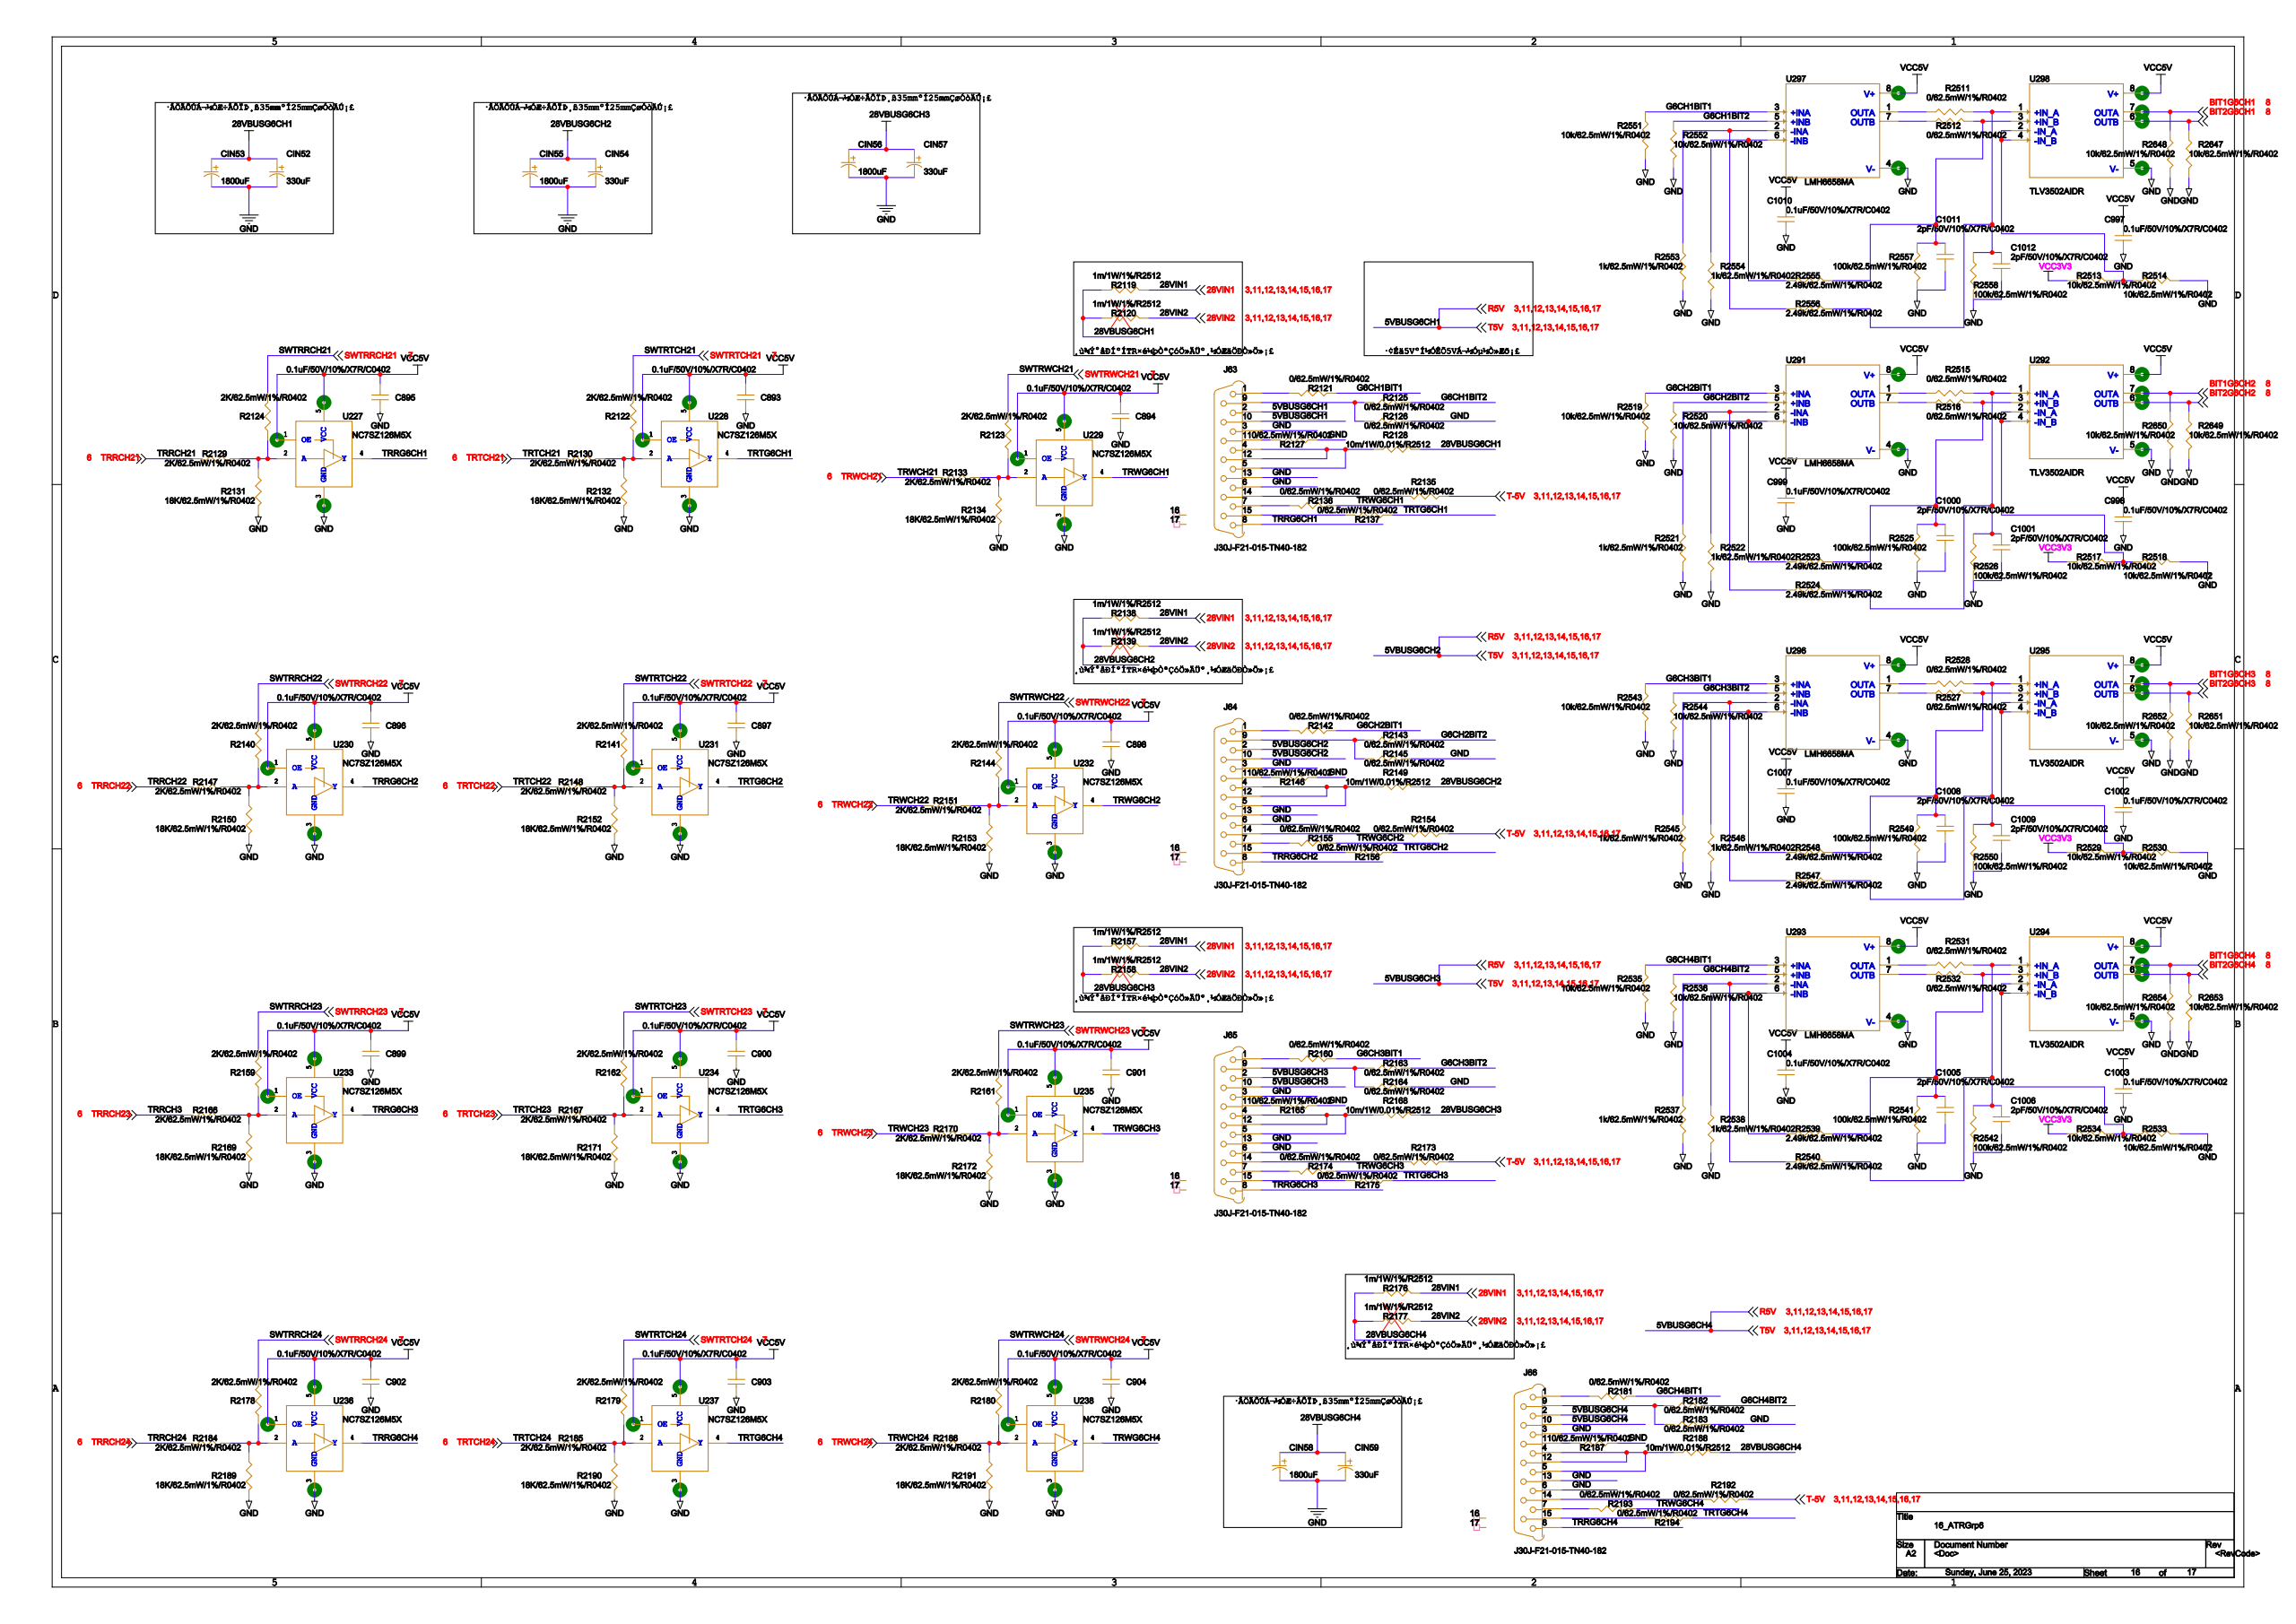Circuit board | Cadence Allegro | 1997 parts | 1536 nets | one sheet of the schematic
Parts on this sheet (reference | value | footprint):
C893 | 0.1uF/50V/10%/X7R/C0402 | 0402
C894 | 0.1uF/50V/10%/X7R/C0402 | 0402
C895 | 0.1uF/50V/10%/X7R/C0402 | 0402
C896 | 0.1uF/50V/10%/X7R/C0402 | 0402
C897 | 0.1uF/50V/10%/X7R/C0402 | 0402
C898 | 0.1uF/50V/10%/X7R/C0402 | 0402
C899 | 0.1uF/50V/10%/X7R/C0402 | 0402
C900 | 0.1uF/50V/10%/X7R/C0402 | 0402
C901 | 0.1uF/50V/10%/X7R/C0402 | 0402
C902 | 0.1uF/50V/10%/X7R/C0402 | 0402
C903 | 0.1uF/50V/10%/X7R/C0402 | 0402
C904 | 0.1uF/50V/10%/X7R/C0402 | 0402
C997 | 0.1uF/50V/10%/X7R/C0402 | 0402
C998 | 0.1uF/50V/10%/X7R/C0402 | 0402
C1000 | 2pF/50V/10%/X7R/C0402 | 0402
C1001 | 2pF/50V/10%/X7R/C0402 | 0402
C1002 | 0.1uF/50V/10%/X7R/C0402 | 0402
C1003 | 0.1uF/50V/10%/X7R/C0402 | 0402
C1005 | 2pF/50V/10%/X7R/C0402 | 0402
C1006 | 2pF/50V/10%/X7R/C0402 | 0402
C1008 | 2pF/50V/10%/X7R/C0402 | 0402
C1009 | 2pF/50V/10%/X7R/C0402 | 0402
C1011 | 2pF/50V/10%/X7R/C0402 | 0402
C1012 | 2pF/50V/10%/X7R/C0402 | 0402
CIN52 | ECF1JM331G20OTPO | AP-SMD_BD10-L20-W6_6-LS7_21
CIN53 | ECF1HM182M27OTPO | AP-SMD_BD18-L27-W6_6-LS7_21
CIN54 | ECF1JM331G20OTPO | AP-SMD_BD10-L20-W6_6-LS7_21
CIN55 | ECF1HM182M27OTPO | AP-SMD_BD18-L27-W6_6-LS7_21
CIN56 | ECF1HM182M27OTPO | AP-SMD_BD18-L27-W6_6-LS7_21
CIN57 | ECF1JM331G20OTPO | AP-SMD_BD10-L20-W6_6-LS7_21
CIN58 | ECF1HM182M27OTPO | AP-SMD_BD18-L27-W6_6-LS7_21
CIN59 | ECF1JM331G20OTPO | AP-SMD_BD10-L20-W6_6-LS7_21
J63 | J30J-F21-015-TN40-182 | J30J-F21-015-TN40-182
J64 | J30J-F21-015-TN40-182 | J30J-F21-015-TN40-182
J65 | J30J-F21-015-TN40-182 | J30J-F21-015-TN40-182
J66 | J30J-F21-015-TN40-182 | J30J-F21-015-TN40-182
R2119 | 1m/1W/1%/R2512 | 2512
R2120 | 1m/1W/1%/R2512 | 2512
R2121 | 0/62.5mW/1%/R0402 | 0402
R2122 | 2K/62.5mW/1%/R0402 | 0402
R2123 | 2K/62.5mW/1%/R0402 | 0402
R2124 | 2K/62.5mW/1%/R0402 | 0402
R2125 | 0/62.5mW/1%/R0402 | 0402
R2126 | 0/62.5mW/1%/R0402 | 0402
R2127 | 0/62.5mW/1%/R0402 | 0402
R2128 | 10m/1W/0.01%/R2512 | 2512
R2129 | 2K/62.5mW/1%/R0402 | 0402
R2130 | 2K/62.5mW/1%/R0402 | 0402
R2131 | 18K/62.5mW/1%/R0402 | 0402
R2132 | 18K/62.5mW/1%/R0402 | 0402
R2133 | 2K/62.5mW/1%/R0402 | 0402
R2134 | 18K/62.5mW/1%/R0402 | 0402
R2135 | 0/62.5mW/1%/R0402 | 0402
R2136 | 0/62.5mW/1%/R0402 | 0402
R2137 | 0/62.5mW/1%/R0402 | 0402
R2138 | 1m/1W/1%/R2512 | 2512
R2139 | 1m/1W/1%/R2512 | 2512
R2140 | 2K/62.5mW/1%/R0402 | 0402
R2141 | 2K/62.5mW/1%/R0402 | 0402
R2142 | 0/62.5mW/1%/R0402 | 0402
R2143 | 0/62.5mW/1%/R0402 | 0402
R2144 | 2K/62.5mW/1%/R0402 | 0402
R2145 | 0/62.5mW/1%/R0402 | 0402
R2146 | 0/62.5mW/1%/R0402 | 0402
R2147 | 2K/62.5mW/1%/R0402 | 0402
R2148 | 2K/62.5mW/1%/R0402 | 0402
R2149 | 10m/1W/0.01%/R2512 | 2512
R2150 | 18K/62.5mW/1%/R0402 | 0402
R2151 | 2K/62.5mW/1%/R0402 | 0402
R2152 | 18K/62.5mW/1%/R0402 | 0402
R2153 | 18K/62.5mW/1%/R0402 | 0402
R2154 | 0/62.5mW/1%/R0402 | 0402
R2155 | 0/62.5mW/1%/R0402 | 0402
R2156 | 0/62.5mW/1%/R0402 | 0402
R2157 | 1m/1W/1%/R2512 | 2512
R2158 | 1m/1W/1%/R2512 | 2512
R2159 | 2K/62.5mW/1%/R0402 | 0402
R2160 | 0/62.5mW/1%/R0402 | 0402
R2161 | 2K/62.5mW/1%/R0402 | 0402
R2162 | 2K/62.5mW/1%/R0402 | 0402
R2163 | 0/62.5mW/1%/R0402 | 0402
R2164 | 0/62.5mW/1%/R0402 | 0402
R2165 | 0/62.5mW/1%/R0402 | 0402
R2166 | 2K/62.5mW/1%/R0402 | 0402
R2167 | 2K/62.5mW/1%/R0402 | 0402
R2168 | 10m/1W/0.01%/R2512 | 2512
R2169 | 18K/62.5mW/1%/R0402 | 0402
R2170 | 2K/62.5mW/1%/R0402 | 0402
R2171 | 18K/62.5mW/1%/R0402 | 0402
R2172 | 18K/62.5mW/1%/R0402 | 0402
R2173 | 0/62.5mW/1%/R0402 | 0402
R2174 | 0/62.5mW/1%/R0402 | 0402
R2175 | 0/62.5mW/1%/R0402 | 0402
R2176 | 1m/1W/1%/R2512 | 2512
R2177 | 1m/1W/1%/R2512 | 2512
R2178 | 2K/62.5mW/1%/R0402 | 0402
R2179 | 2K/62.5mW/1%/R0402 | 0402
R2180 | 2K/62.5mW/1%/R0402 | 0402
R2181 | 0/62.5mW/1%/R0402 | 0402
R2182 | 0/62.5mW/1%/R0402 | 0402
R2183 | 0/62.5mW/1%/R0402 | 0402
R2184 | 2K/62.5mW/1%/R0402 | 0402
R2185 | 2K/62.5mW/1%/R0402 | 0402
R2186 | 2K/62.5mW/1%/R0402 | 0402
R2187 | 0/62.5mW/1%/R0402 | 0402
R2188 | 10m/1W/0.01%/R2512 | 2512
R2189 | 18K/62.5mW/1%/R0402 | 0402
R2190 | 18K/62.5mW/1%/R0402 | 0402
R2191 | 18K/62.5mW/1%/R0402 | 0402
R2192 | 0/62.5mW/1%/R0402 | 0402
R2193 | 0/62.5mW/1%/R0402 | 0402
R2194 | 0/62.5mW/1%/R0402 | 0402
R2511 | 0/62.5mW/1%/R0402 | 0402
R2512 | 0/62.5mW/1%/R0402 | 0402
R2513 | 10k/62.5mW/1%/R0402 | 0402
R2514 | 10k/62.5mW/1%/R0402 | 0402
R2515 | 0/62.5mW/1%/R0402 | 0402
R2516 | 0/62.5mW/1%/R0402 | 0402
R2517 | 10k/62.5mW/1%/R0402 | 0402
R2518 | 10k/62.5mW/1%/R0402 | 0402
R2519 | 10k/62.5mW/1%/R0402 | 0402
R2520 | 10k/62.5mW/1%/R0402 | 0402
R2521 | 1K/62.5mW/1%/R0402 | 0402
R2522 | 1K/62.5mW/1%/R0402 | 0402
R2524 | 2.49k/62.5mW/1%/R0402 | 0402
R2525 | 100k/62.5mW/1%/R0402 | 0402
R2526 | 100k/62.5mW/1%/R0402 | 0402
R2527 | 0/62.5mW/1%/R0402 | 0402
R2528 | 0/62.5mW/1%/R0402 | 0402
R2529 | 10k/62.5mW/1%/R0402 | 0402
R2530 | 10k/62.5mW/1%/R0402 | 0402
R2531 | 0/62.5mW/1%/R0402 | 0402
R2532 | 0/62.5mW/1%/R0402 | 0402
R2533 | 10k/62.5mW/1%/R0402 | 0402
R2534 | 10k/62.5mW/1%/R0402 | 0402
R2535 | 10k/62.5mW/1%/R0402 | 0402
R2536 | 10k/62.5mW/1%/R0402 | 0402
R2537 | 1K/62.5mW/1%/R0402 | 0402
R2538 | 1K/62.5mW/1%/R0402 | 0402
R2540 | 2.49k/62.5mW/1%/R0402 | 0402
R2541 | 100k/62.5mW/1%/R0402 | 0402
R2542 | 100k/62.5mW/1%/R0402 | 0402
R2543 | 10k/62.5mW/1%/R0402 | 0402
R2544 | 10k/62.5mW/1%/R0402 | 0402
R2545 | 1K/62.5mW/1%/R0402 | 0402
R2546 | 1K/62.5mW/1%/R0402 | 0402
R2547 | 2.49k/62.5mW/1%/R0402 | 0402
R2548 | 2.49k/62.5mW/1%/R0402 | 0402
R2549 | 100k/62.5mW/1%/R0402 | 0402
R2550 | 100k/62.5mW/1%/R0402 | 0402
R2551 | 10k/62.5mW/1%/R0402 | 0402
R2552 | 10k/62.5mW/1%/R0402 | 0402
R2553 | 1K/62.5mW/1%/R0402 | 0402
R2554 | 1K/62.5mW/1%/R0402 | 0402
R2556 | 2.49k/62.5mW/1%/R0402 | 0402
R2557 | 100k/62.5mW/1%/R0402 | 0402
R2558 | 100k/62.5mW/1%/R0402 | 0402
R2647 | 10k/62.5mW/1%/R0402 | 0402
R2648 | 10k/62.5mW/1%/R0402 | 0402
R2649 | 10k/62.5mW/1%/R0402 | 0402
R2650 | 10k/62.5mW/1%/R0402 | 0402
R2651 | 10k/62.5mW/1%/R0402 | 0402
R2652 | 10k/62.5mW/1%/R0402 | 0402
R2653 | 10k/62.5mW/1%/R0402 | 0402
R2654 | 10k/62.5mW/1%/R0402 | 0402
U227 | NC7SZ126M5X | SOT-23-5
U228 | NC7SZ126M5X | SOT-23-5
U229 | NC7SZ126M5X | SOT-23-5
U230 | NC7SZ126M5X | SOT-23-5
U231 | NC7SZ126M5X | SOT-23-5
U232 | NC7SZ126M5X | SOT-23-5
U233 | NC7SZ126M5X | SOT-23-5
U234 | NC7SZ126M5X | SOT-23-5
U235 | NC7SZ126M5X | SOT-23-5
U236 | NC7SZ126M5X | SOT-23-5
U237 | NC7SZ126M5X | SOT-23-5
U238 | NC7SZ126M5X | SOT-23-5
U291 | LMH6658MA | SOIC127P599X175-8N
U293 | LMH6658MA | SOIC127P599X175-8N
U295 | TLV3502AIDR | SOIC127P599X175-8N
U297 | LMH6658MA | SOIC127P599X175-8N
Nets of these parts (net: part-pin ...):
3.3V: R2513-1 R2517-1 R2529-1 R2534-1
AGND: C893-2 C894-2 C895-2 C896-2 C897-2 C898-2 C899-2 C900-2 C901-2 C902-2 C903-2 C904-2 C997-2 C998-2 C1000-2 C1001-2 C1002-2 C1003-2 C1005-2 C1006-2 C1008-2 C1009-2 C1011-2 C1012-2 CIN52-2 CIN53-2 CIN54-2 CIN55-2 CIN56-2 CIN57-2 CIN58-2 CIN59-2 J63-3 J63-6 J63-13 J64-3 J64-6 J64-13 J65-3 J65-6 J65-13 J66-3 J66-6 J66-13 R2126-1 R2127-1 R2131-1 R2132-1 R2134-1 R2145-1 R2146-1 R2150-1 R2152-1 R2153-1 R2164-1 R2165-1 R2169-1 R2171-1 R2172-1 R2183-1 R2187-1 R2189-1 R2190-1 R2191-1 R2514-2 R2518-2 R2519-2 R2520-2 R2521-2 R2522-2 R2525-2 R2526-2 R2530-2 R2533-2 R2535-2 R2536-2 R2537-2 R2538-2 R2541-2 R2542-2 R2543-2 R2544-2 R2545-2 R2546-2 R2549-2 R2550-2 R2551-2 R2552-2 R2553-2 R2554-2 R2557-2 R2558-2 R2647-2 R2648-2 R2649-2 R2650-2 R2651-2 R2652-2 R2653-2 R2654-2 U227-3 U228-3 U229-3 U230-3 U231-3 U232-3 U233-3 U234-3 U235-3 U236-3 U237-3 U238-3 U291-4 U293-4 U295-5 U297-4
VCC5V: C893-1 C894-1 C895-1 C896-1 C897-1 C898-1 C899-1 C900-1 C901-1 C902-1 C903-1 C904-1 C997-1 C998-1 C1002-1 C1003-1 U227-1 U227-5 U228-1 U228-5 U229-1 U229-5 U230-1 U230-5 U231-1 U231-5 U232-1 U232-5 U233-1 U233-5 U234-1 U234-5 U235-1 U235-5 U236-1 U236-5 U237-1 U237-5 U238-1 U238-5 U291-8 U293-8 U295-8 U297-8
N24409583: R2522-1 U291-6
N24409593: C1000-1 R2516-2 R2525-1
N24409571: R2521-1 R2524-1 U291-2
N24409591: C1001-1 R2515-2 R2524-2 R2526-1
N24410137: R2538-1 U293-6
N24410147: C1005-1 R2532-2 R2541-1
N24410125: R2537-1 R2540-1 U293-2
N24410145: C1006-1 R2531-2 R2540-2 R2542-1
N24409949: R2545-1 R2547-1
N24409965: C1009-1 R2528-2 R2547-2 R2550-1 U295-1
N24409953: R2546-1 R2548-1
N24409967: C1008-1 R2527-2 R2548-2 R2549-1 U295-3
N24409403: R2554-1 U297-6
N24409413: C1011-1 R2512-2 R2557-1
N24409399: R2553-1 R2556-1 U297-2
N24409411: C1012-1 R2511-2 R2556-2 R2558-1
G6CH2BIT1: R2142-1 R2519-1 U291-3
G6CH2BIT2: R2143-1 R2520-1 U291-5
N24409587: R2515-1 U291-1
N24409589: R2516-1 U291-7
G6CH4BIT1: R2181-1 R2535-1 U293-3
G6CH4BIT2: R2182-1 R2536-1 U293-5
N24410141: R2531-1 U293-1
N24410143: R2532-1 U293-7
G6CH3BIT1: R2160-1 R2543-1
G6CH3BIT2: R2163-1 R2544-1
N24409961: R2528-1
N24409963: R2527-1
G6CH1BIT1: R2121-1 R2551-1 U297-3
G6CH1BIT2: R2125-1 R2552-1 U297-5
N24409407: R2511-1 U297-1
N24409409: R2512-1 U297-7
N24409645: R2517-2 R2518-1
BIT1G6CH2: R2650-1
BIT2G6CH2: R2649-1
N24410199: R2533-1 R2534-2
BIT1G6CH4: R2654-1
BIT2G6CH4: R2653-1
N24410019: R2529-2 R2530-1 U295-2 U295-4
BIT1G6CH3: R2652-1 U295-7
BIT2G6CH3: R2651-1 U295-6
N24409465: R2513-2 R2514-1
BIT1G6CH1: R2648-1
BIT2G6CH1: R2647-1
R5V: J63-2 J63-10 J64-2 J64-10 J65-2 J65-10 J66-2 J66-10
N23733637: J63-1 R2121-2
N23733650: J63-11 R2127-2
N23733652: J63-4 J63-5 J63-12 R2128-1
N23733664: J63-14 R2135-2
N23733668: J63-15 R2137-2
N23733666: J63-7 R2136-2
TRRG6CH1: J63-8 U227-4
N23733639: J63-9 R2125-2 R2126-2
N23734196: J64-1 R2142-2
N23734209: J64-11 R2146-2
N23734211: J64-4 J64-5 J64-12 R2149-1
N23734223: J64-14 R2154-2
N23734227: J64-15 R2156-2
N23734225: J64-7 R2155-2
TRRG6CH2: J64-8 U230-4
N23734198: J64-9 R2143-2 R2145-2
N23734823: J65-1 R2160-2
N23734836: J65-11 R2165-2
N23734838: J65-4 J65-5 J65-12 R2168-1
N23734850: J65-14 R2173-2
N23734854: J65-15 R2175-2
N23734852: J65-7 R2174-2
TRRG6CH3: J65-8 U233-4
N23734825: J65-9 R2163-2 R2164-2
N23735455: J66-1 R2181-2
N23735468: J66-11 R2187-2
N23735470: J66-4 J66-5 J66-12 R2188-1
N23735482: J66-14 R2192-2
N23735486: J66-15 R2194-2
N23735484: J66-7 R2193-2
TRRG6CH4: J66-8 U236-4
N23735457: J66-9 R2182-2 R2183-2
28VIN1: R2119-2 R2138-2 R2157-2 R2176-2
T-5V: R2135-1 R2154-1 R2173-1 R2192-1
28VIN2: R2120-2 R2139-2 R2158-2 R2177-2
28VBUSG6CH1: CIN52-1 CIN53-1 R2119-1 R2120-1 R2128-2
28VBUSG6CH2: CIN54-1 CIN55-1 R2138-1 R2139-1 R2149-2
28VBUSG6CH3: CIN56-1 CIN57-1 R2157-1 R2158-1 R2168-2
28VBUSG6CH4: CIN58-1 CIN59-1 R2176-1 R2177-1 R2188-2
SWTRTCH21: R2122-1
N24017305: R2122-2 R2130-2 R2132-2 U228-2
SWTRWCH21: R2123-1
N24017793: R2123-2 R2133-2 R2134-2 U229-2
SWTRRCH21: R2124-1
N24018285: R2124-2 R2129-2 R2131-2 U227-2
TRRCH21: R2129-1
TRTCH21: R2130-1
TRWCH21: R2133-1
SWTRRCH22: R2140-1
N24018403: R2140-2 R2147-2 R2150-2 U230-2
SWTRTCH22: R2141-1
N24017423: R2141-2 R2148-2 R2152-2 U231-2
SWTRWCH22: R2144-1
N24017915: R2144-2 R2151-2 R2153-2 U232-2
TRRCH22: R2147-1
TRTCH22: R2148-1
TRWCH22: R2151-1
SWTRRCH23: R2159-1
N24018529: R2159-2 R2166-2 R2169-2 U233-2
SWTRWCH23: R2161-1
N24018037: R2161-2 R2170-2 R2172-2 U235-2
SWTRTCH23: R2162-1
N24017549: R2162-2 R2167-2 R2171-2 U234-2
TRRCH23: R2166-1
TRTCH23: R2167-1
TRWCH23: R2170-1
SWTRRCH24: R2178-1
N24018647: R2178-2 R2184-2 R2189-2 U236-2
SWTRTCH24: R2179-1
N24017671: R2179-2 R2185-2 R2190-2 U237-2
SWTRWCH24: R2180-1
N24018159: R2180-2 R2186-2 R2191-2 U238-2
TRRCH24: R2184-1
TRTCH24: R2185-1
TRWCH24: R2186-1
TRTG6CH1: R2137-1 U228-4
TRWG6CH1: R2136-1 U229-4
TRTG6CH2: R2156-1 U231-4
TRWG6CH2: R2155-1 U232-4
TRTG6CH3: R2175-1 U234-4
TRWG6CH3: R2174-1 U235-4
TRTG6CH4: R2194-1 U237-4
TRWG6CH4: R2193-1 U238-4